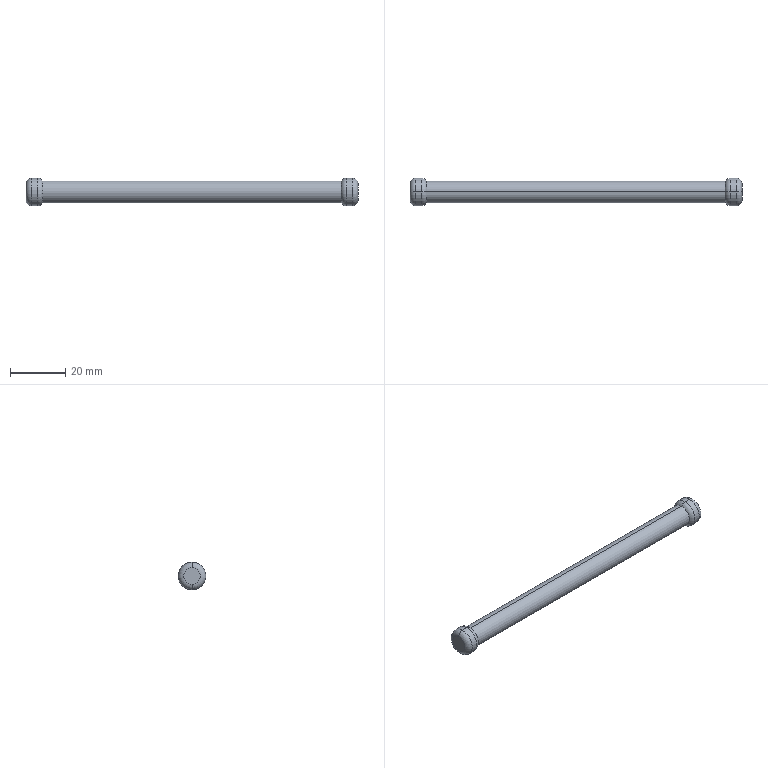Part | SolidWorks | features Fillet 1, ICE 1, MirrorPattern 1, Revolution 1 | 1 solid | 16 faces | box 120 x 10 x 10 mm | volume 6156 mm3 | torus 8 | cylinder 6 | plane 2 | commonest cylinder face diameters 10 x4 7.9 x2
STEP:
#1=CARTESIAN_POINT('',(84.907,0.,-5.));
#2=VERTEX_POINT('',#1);
#3=CARTESIAN_POINT('',(84.907,0.,5.));
#4=VERTEX_POINT('',#3);
#5=CARTESIAN_POINT('',(84.907,0.,0.));
#6=DIRECTION('',(1.,0.,0.));
#7=DIRECTION('',(0.,0.,1.));
#8=AXIS2_PLACEMENT_3D('',#5,#6,#7);
#9=CIRCLE('',#8,5.);
#10=EDGE_CURVE('',#2,#4,#9,.T.);
#11=ORIENTED_EDGE('',*,*,#10,.F.);
#12=CARTESIAN_POINT('',(83.147,0.,-3.95));
#13=VERTEX_POINT('',#12);
#14=CARTESIAN_POINT('',(84.907,0.,-3.));
#15=DIRECTION('',(0.,1.,0.));
#16=DIRECTION('',(0.,0.,1.));
#17=AXIS2_PLACEMENT_3D('',#14,#15,#16);
#18=CIRCLE('',#17,2.);
#19=EDGE_CURVE('',#2,#13,#18,.T.);
#20=ORIENTED_EDGE('',*,*,#19,.T.);
#21=CARTESIAN_POINT('',(83.147,0.,3.95));
#22=VERTEX_POINT('',#21);
#23=CARTESIAN_POINT('',(83.147,0.,0.));
#24=DIRECTION('',(1.,0.,0.));
#25=DIRECTION('',(0.,0.,-1.));
#26=AXIS2_PLACEMENT_3D('',#23,#24,#25);
#27=CIRCLE('',#26,3.95);
#28=EDGE_CURVE('',#13,#22,#27,.T.);
#29=ORIENTED_EDGE('',*,*,#28,.T.);
#30=CARTESIAN_POINT('',(84.907,0.,3.));
#31=DIRECTION('',(0.,-1.,0.));
#32=DIRECTION('',(0.,0.,-1.));
#33=AXIS2_PLACEMENT_3D('',#30,#31,#32);
#34=CIRCLE('',#33,2.);
#35=EDGE_CURVE('',#4,#22,#34,.T.);
#36=ORIENTED_EDGE('',*,*,#35,.F.);
#37=EDGE_LOOP('',(#11,#20,#29,#36));
#38=FACE_OUTER_BOUND('',#37,.T.);
#39=CARTESIAN_POINT('',(84.907,0.,0.));
#40=DIRECTION('',(-1.,0.,0.));
#41=DIRECTION('',(0.,0.,1.));
#42=AXIS2_PLACEMENT_3D('',#39,#40,#41);
#43=TOROIDAL_SURFACE('',#42,3.,2.);
#44=ADVANCED_FACE('',(#38),#43,.T.);
#45=CARTESIAN_POINT('',(89.147,0.,-3.));
#46=VERTEX_POINT('',#45);
#47=CARTESIAN_POINT('',(89.147,0.,3.));
#48=VERTEX_POINT('',#47);
#49=CARTESIAN_POINT('',(89.147,0.,0.));
#50=DIRECTION('',(1.,0.,0.));
#51=DIRECTION('',(0.,0.,1.));
#52=AXIS2_PLACEMENT_3D('',#49,#50,#51);
#53=CIRCLE('',#52,3.);
#54=EDGE_CURVE('',#46,#48,#53,.T.);
#55=ORIENTED_EDGE('',*,*,#54,.F.);
#56=CARTESIAN_POINT('',(87.147,0.,-5.));
#57=VERTEX_POINT('',#56);
#58=CARTESIAN_POINT('',(87.147,0.,-3.));
#59=DIRECTION('',(0.,1.,0.));
#60=DIRECTION('',(0.,0.,1.));
#61=AXIS2_PLACEMENT_3D('',#58,#59,#60);
#62=CIRCLE('',#61,2.);
#63=EDGE_CURVE('',#46,#57,#62,.T.);
#64=ORIENTED_EDGE('',*,*,#63,.T.);
#65=CARTESIAN_POINT('',(87.147,0.,5.));
#66=VERTEX_POINT('',#65);
#67=CARTESIAN_POINT('',(87.147,0.,0.));
#68=DIRECTION('',(-1.,0.,0.));
#69=DIRECTION('',(0.,0.,1.));
#70=AXIS2_PLACEMENT_3D('',#67,#68,#69);
#71=CIRCLE('',#70,5.);
#72=EDGE_CURVE('',#66,#57,#71,.T.);
#73=ORIENTED_EDGE('',*,*,#72,.F.);
#74=CARTESIAN_POINT('',(87.147,0.,3.));
#75=DIRECTION('',(0.,-1.,0.));
#76=DIRECTION('',(0.,0.,-1.));
#77=AXIS2_PLACEMENT_3D('',#74,#75,#76);
#78=CIRCLE('',#77,2.);
#79=EDGE_CURVE('',#48,#66,#78,.T.);
#80=ORIENTED_EDGE('',*,*,#79,.F.);
#81=EDGE_LOOP('',(#55,#64,#73,#80));
#82=FACE_OUTER_BOUND('',#81,.T.);
#83=CARTESIAN_POINT('',(87.147,0.,0.));
#84=DIRECTION('',(-1.,0.,0.));
#85=DIRECTION('',(0.,0.,1.));
#86=AXIS2_PLACEMENT_3D('',#83,#84,#85);
#87=TOROIDAL_SURFACE('',#86,3.,2.);
#88=ADVANCED_FACE('',(#82),#87,.T.);
#89=ORIENTED_EDGE('',*,*,#10,.T.);
#90=CARTESIAN_POINT('',(83.147,0.,5.));
#91=DIRECTION('',(1.,0.,0.));
#92=VECTOR('',#91,1000.);
#93=LINE('',#90,#92);
#94=EDGE_CURVE('',#4,#66,#93,.T.);
#95=ORIENTED_EDGE('',*,*,#94,.T.);
#96=ORIENTED_EDGE('',*,*,#72,.T.);
#97=CARTESIAN_POINT('',(83.147,0.,-5.));
#98=DIRECTION('',(1.,0.,0.));
#99=VECTOR('',#98,1000.);
#100=LINE('',#97,#99);
#101=EDGE_CURVE('',#2,#57,#100,.T.);
#102=ORIENTED_EDGE('',*,*,#101,.F.);
#103=EDGE_LOOP('',(#89,#95,#96,#102));
#104=FACE_OUTER_BOUND('',#103,.T.);
#105=CARTESIAN_POINT('',(83.147,0.,0.));
#106=DIRECTION('',(1.,0.,0.));
#107=DIRECTION('',(0.,0.,-1.));
#108=AXIS2_PLACEMENT_3D('',#105,#106,#107);
#109=CYLINDRICAL_SURFACE('',#108,5.);
#110=ADVANCED_FACE('',(#104),#109,.T.);
#111=CARTESIAN_POINT('',(-26.613,0.,5.));
#112=VERTEX_POINT('',#111);
#113=CARTESIAN_POINT('',(-26.613,0.,-5.));
#114=VERTEX_POINT('',#113);
#115=CARTESIAN_POINT('',(-26.613,0.,0.));
#116=DIRECTION('',(-1.,0.,0.));
#117=DIRECTION('',(0.,0.,-1.));
#118=AXIS2_PLACEMENT_3D('',#115,#116,#117);
#119=CIRCLE('',#118,5.);
#120=EDGE_CURVE('',#112,#114,#119,.T.);
#121=ORIENTED_EDGE('',*,*,#120,.F.);
#122=CARTESIAN_POINT('',(-24.853,0.,3.95));
#123=VERTEX_POINT('',#122);
#124=CARTESIAN_POINT('',(-26.613,0.,3.));
#125=DIRECTION('',(0.,1.,0.));
#126=DIRECTION('',(0.,0.,1.));
#127=AXIS2_PLACEMENT_3D('',#124,#125,#126);
#128=CIRCLE('',#127,2.);
#129=EDGE_CURVE('',#112,#123,#128,.T.);
#130=ORIENTED_EDGE('',*,*,#129,.T.);
#131=CARTESIAN_POINT('',(-24.853,0.,-3.95));
#132=VERTEX_POINT('',#131);
#133=CARTESIAN_POINT('',(-24.853,0.,0.));
#134=DIRECTION('',(-1.,0.,0.));
#135=DIRECTION('',(0.,0.,1.));
#136=AXIS2_PLACEMENT_3D('',#133,#134,#135);
#137=CIRCLE('',#136,3.95);
#138=EDGE_CURVE('',#123,#132,#137,.T.);
#139=ORIENTED_EDGE('',*,*,#138,.T.);
#140=CARTESIAN_POINT('',(-26.613,0.,-3.));
#141=DIRECTION('',(0.,-1.,0.));
#142=DIRECTION('',(0.,0.,-1.));
#143=AXIS2_PLACEMENT_3D('',#140,#141,#142);
#144=CIRCLE('',#143,2.);
#145=EDGE_CURVE('',#114,#132,#144,.T.);
#146=ORIENTED_EDGE('',*,*,#145,.F.);
#147=EDGE_LOOP('',(#121,#130,#139,#146));
#148=FACE_OUTER_BOUND('',#147,.T.);
#149=CARTESIAN_POINT('',(-26.613,0.,0.));
#150=DIRECTION('',(1.,0.,0.));
#151=DIRECTION('',(0.,0.,-1.));
#152=AXIS2_PLACEMENT_3D('',#149,#150,#151);
#153=TOROIDAL_SURFACE('',#152,3.,2.);
#154=ADVANCED_FACE('',(#148),#153,.T.);
#155=CARTESIAN_POINT('',(-30.853,0.,3.));
#156=VERTEX_POINT('',#155);
#157=CARTESIAN_POINT('',(-30.853,0.,-3.));
#158=VERTEX_POINT('',#157);
#159=CARTESIAN_POINT('',(-30.853,0.,0.));
#160=DIRECTION('',(-1.,0.,0.));
#161=DIRECTION('',(0.,0.,-1.));
#162=AXIS2_PLACEMENT_3D('',#159,#160,#161);
#163=CIRCLE('',#162,3.);
#164=EDGE_CURVE('',#156,#158,#163,.T.);
#165=ORIENTED_EDGE('',*,*,#164,.F.);
#166=CARTESIAN_POINT('',(-28.853,0.,5.));
#167=VERTEX_POINT('',#166);
#168=CARTESIAN_POINT('',(-28.853,0.,3.));
#169=DIRECTION('',(0.,1.,0.));
#170=DIRECTION('',(0.,0.,1.));
#171=AXIS2_PLACEMENT_3D('',#168,#169,#170);
#172=CIRCLE('',#171,2.);
#173=EDGE_CURVE('',#156,#167,#172,.T.);
#174=ORIENTED_EDGE('',*,*,#173,.T.);
#175=CARTESIAN_POINT('',(-28.853,0.,-5.));
#176=VERTEX_POINT('',#175);
#177=CARTESIAN_POINT('',(-28.853,0.,0.));
#178=DIRECTION('',(1.,0.,0.));
#179=DIRECTION('',(0.,0.,-1.));
#180=AXIS2_PLACEMENT_3D('',#177,#178,#179);
#181=CIRCLE('',#180,5.);
#182=EDGE_CURVE('',#176,#167,#181,.T.);
#183=ORIENTED_EDGE('',*,*,#182,.F.);
#184=CARTESIAN_POINT('',(-28.853,0.,-3.));
#185=DIRECTION('',(0.,-1.,0.));
#186=DIRECTION('',(0.,0.,-1.));
#187=AXIS2_PLACEMENT_3D('',#184,#185,#186);
#188=CIRCLE('',#187,2.);
#189=EDGE_CURVE('',#158,#176,#188,.T.);
#190=ORIENTED_EDGE('',*,*,#189,.F.);
#191=EDGE_LOOP('',(#165,#174,#183,#190));
#192=FACE_OUTER_BOUND('',#191,.T.);
#193=CARTESIAN_POINT('',(-28.853,0.,0.));
#194=DIRECTION('',(1.,0.,0.));
#195=DIRECTION('',(0.,0.,-1.));
#196=AXIS2_PLACEMENT_3D('',#193,#194,#195);
#197=TOROIDAL_SURFACE('',#196,3.,2.);
#198=ADVANCED_FACE('',(#192),#197,.T.);
#199=ORIENTED_EDGE('',*,*,#120,.T.);
#200=CARTESIAN_POINT('',(-24.853,0.,-5.));
#201=DIRECTION('',(-1.,0.,0.));
#202=VECTOR('',#201,1000.);
#203=LINE('',#200,#202);
#204=EDGE_CURVE('',#114,#176,#203,.T.);
#205=ORIENTED_EDGE('',*,*,#204,.T.);
#206=ORIENTED_EDGE('',*,*,#182,.T.);
#207=CARTESIAN_POINT('',(-24.853,0.,5.));
#208=DIRECTION('',(-1.,0.,0.));
#209=VECTOR('',#208,1000.);
#210=LINE('',#207,#209);
#211=EDGE_CURVE('',#112,#167,#210,.T.);
#212=ORIENTED_EDGE('',*,*,#211,.F.);
#213=EDGE_LOOP('',(#199,#205,#206,#212));
#214=FACE_OUTER_BOUND('',#213,.T.);
#215=CARTESIAN_POINT('',(-24.853,0.,0.));
#216=DIRECTION('',(-1.,0.,0.));
#217=DIRECTION('',(0.,0.,1.));
#218=AXIS2_PLACEMENT_3D('',#215,#216,#217);
#219=CYLINDRICAL_SURFACE('',#218,5.);
#220=ADVANCED_FACE('',(#214),#219,.T.);
#221=ORIENTED_EDGE('',*,*,#28,.F.);
#222=CARTESIAN_POINT('',(-30.853,0.,-3.95));
#223=DIRECTION('',(-1.,0.,0.));
#224=VECTOR('',#223,1000.);
#225=LINE('',#222,#224);
#226=EDGE_CURVE('',#13,#132,#225,.T.);
#227=ORIENTED_EDGE('',*,*,#226,.T.);
#228=ORIENTED_EDGE('',*,*,#138,.F.);
#229=CARTESIAN_POINT('',(-30.853,0.,3.95));
#230=DIRECTION('',(-1.,0.,0.));
#231=VECTOR('',#230,1000.);
#232=LINE('',#229,#231);
#233=EDGE_CURVE('',#22,#123,#232,.T.);
#234=ORIENTED_EDGE('',*,*,#233,.F.);
#235=EDGE_LOOP('',(#221,#227,#228,#234));
#236=FACE_OUTER_BOUND('',#235,.T.);
#237=CARTESIAN_POINT('',(-30.853,0.,0.));
#238=DIRECTION('',(-1.,0.,0.));
#239=DIRECTION('',(0.,0.,1.));
#240=AXIS2_PLACEMENT_3D('',#237,#238,#239);
#241=CYLINDRICAL_SURFACE('',#240,3.95);
#242=ADVANCED_FACE('',(#236),#241,.T.);
#243=ORIENTED_EDGE('',*,*,#226,.F.);
#244=CARTESIAN_POINT('',(83.147,0.,0.));
#245=DIRECTION('',(1.,0.,0.));
#246=DIRECTION('',(0.,0.,-1.));
#247=AXIS2_PLACEMENT_3D('',#244,#245,#246);
#248=CIRCLE('',#247,3.95);
#249=EDGE_CURVE('',#22,#13,#248,.T.);
#250=ORIENTED_EDGE('',*,*,#249,.F.);
#251=ORIENTED_EDGE('',*,*,#233,.T.);
#252=CARTESIAN_POINT('',(-24.853,0.,0.));
#253=DIRECTION('',(-1.,0.,0.));
#254=DIRECTION('',(0.,0.,1.));
#255=AXIS2_PLACEMENT_3D('',#252,#253,#254);
#256=CIRCLE('',#255,3.95);
#257=EDGE_CURVE('',#132,#123,#256,.T.);
#258=ORIENTED_EDGE('',*,*,#257,.F.);
#259=EDGE_LOOP('',(#243,#250,#251,#258));
#260=FACE_OUTER_BOUND('',#259,.T.);
#261=CARTESIAN_POINT('',(-30.853,0.,0.));
#262=DIRECTION('',(-1.,0.,0.));
#263=DIRECTION('',(0.,0.,1.));
#264=AXIS2_PLACEMENT_3D('',#261,#262,#263);
#265=CYLINDRICAL_SURFACE('',#264,3.95);
#266=ADVANCED_FACE('',(#260),#265,.T.);
#267=ORIENTED_EDGE('',*,*,#204,.F.);
#268=CARTESIAN_POINT('',(-26.613,0.,0.));
#269=DIRECTION('',(-1.,0.,0.));
#270=DIRECTION('',(0.,0.,-1.));
#271=AXIS2_PLACEMENT_3D('',#268,#269,#270);
#272=CIRCLE('',#271,5.);
#273=EDGE_CURVE('',#114,#112,#272,.T.);
#274=ORIENTED_EDGE('',*,*,#273,.T.);
#275=ORIENTED_EDGE('',*,*,#211,.T.);
#276=CARTESIAN_POINT('',(-28.853,0.,0.));
#277=DIRECTION('',(1.,0.,0.));
#278=DIRECTION('',(0.,0.,-1.));
#279=AXIS2_PLACEMENT_3D('',#276,#277,#278);
#280=CIRCLE('',#279,5.);
#281=EDGE_CURVE('',#167,#176,#280,.T.);
#282=ORIENTED_EDGE('',*,*,#281,.T.);
#283=EDGE_LOOP('',(#267,#274,#275,#282));
#284=FACE_OUTER_BOUND('',#283,.T.);
#285=CARTESIAN_POINT('',(-24.853,0.,0.));
#286=DIRECTION('',(-1.,0.,0.));
#287=DIRECTION('',(0.,0.,1.));
#288=AXIS2_PLACEMENT_3D('',#285,#286,#287);
#289=CYLINDRICAL_SURFACE('',#288,5.);
#290=ADVANCED_FACE('',(#284),#289,.T.);
#291=CARTESIAN_POINT('',(-30.853,0.,0.));
#292=DIRECTION('',(-1.,0.,0.));
#293=DIRECTION('',(0.,0.,-1.));
#294=AXIS2_PLACEMENT_3D('',#291,#292,#293);
#295=CIRCLE('',#294,3.);
#296=EDGE_CURVE('',#158,#156,#295,.T.);
#297=ORIENTED_EDGE('',*,*,#296,.T.);
#298=ORIENTED_EDGE('',*,*,#164,.T.);
#299=EDGE_LOOP('',(#297,#298));
#300=FACE_OUTER_BOUND('',#299,.T.);
#301=CARTESIAN_POINT('',(-30.853,0.,0.));
#302=DIRECTION('',(1.,0.,0.));
#303=DIRECTION('',(0.,0.,-1.));
#304=AXIS2_PLACEMENT_3D('',#301,#302,#303);
#305=PLANE('',#304);
#306=ADVANCED_FACE('',(#300),#305,.F.);
#307=ORIENTED_EDGE('',*,*,#173,.F.);
#308=ORIENTED_EDGE('',*,*,#296,.F.);
#309=ORIENTED_EDGE('',*,*,#189,.T.);
#310=ORIENTED_EDGE('',*,*,#281,.F.);
#311=EDGE_LOOP('',(#307,#308,#309,#310));
#312=FACE_OUTER_BOUND('',#311,.T.);
#313=CARTESIAN_POINT('',(-28.853,0.,0.));
#314=DIRECTION('',(1.,0.,0.));
#315=DIRECTION('',(0.,0.,-1.));
#316=AXIS2_PLACEMENT_3D('',#313,#314,#315);
#317=TOROIDAL_SURFACE('',#316,3.,2.);
#318=ADVANCED_FACE('',(#312),#317,.T.);
#319=ORIENTED_EDGE('',*,*,#129,.F.);
#320=ORIENTED_EDGE('',*,*,#273,.F.);
#321=ORIENTED_EDGE('',*,*,#145,.T.);
#322=ORIENTED_EDGE('',*,*,#257,.T.);
#323=EDGE_LOOP('',(#319,#320,#321,#322));
#324=FACE_OUTER_BOUND('',#323,.T.);
#325=CARTESIAN_POINT('',(-26.613,0.,0.));
#326=DIRECTION('',(1.,0.,0.));
#327=DIRECTION('',(0.,0.,-1.));
#328=AXIS2_PLACEMENT_3D('',#325,#326,#327);
#329=TOROIDAL_SURFACE('',#328,3.,2.);
#330=ADVANCED_FACE('',(#324),#329,.T.);
#331=ORIENTED_EDGE('',*,*,#94,.F.);
#332=CARTESIAN_POINT('',(84.907,0.,0.));
#333=DIRECTION('',(1.,0.,0.));
#334=DIRECTION('',(0.,0.,1.));
#335=AXIS2_PLACEMENT_3D('',#332,#333,#334);
#336=CIRCLE('',#335,5.);
#337=EDGE_CURVE('',#4,#2,#336,.T.);
#338=ORIENTED_EDGE('',*,*,#337,.T.);
#339=ORIENTED_EDGE('',*,*,#101,.T.);
#340=CARTESIAN_POINT('',(87.147,0.,0.));
#341=DIRECTION('',(-1.,0.,0.));
#342=DIRECTION('',(0.,0.,1.));
#343=AXIS2_PLACEMENT_3D('',#340,#341,#342);
#344=CIRCLE('',#343,5.);
#345=EDGE_CURVE('',#57,#66,#344,.T.);
#346=ORIENTED_EDGE('',*,*,#345,.T.);
#347=EDGE_LOOP('',(#331,#338,#339,#346));
#348=FACE_OUTER_BOUND('',#347,.T.);
#349=CARTESIAN_POINT('',(83.147,0.,0.));
#350=DIRECTION('',(1.,0.,0.));
#351=DIRECTION('',(0.,0.,-1.));
#352=AXIS2_PLACEMENT_3D('',#349,#350,#351);
#353=CYLINDRICAL_SURFACE('',#352,5.);
#354=ADVANCED_FACE('',(#348),#353,.T.);
#355=CARTESIAN_POINT('',(89.147,0.,0.));
#356=DIRECTION('',(1.,0.,0.));
#357=DIRECTION('',(0.,0.,1.));
#358=AXIS2_PLACEMENT_3D('',#355,#356,#357);
#359=CIRCLE('',#358,3.);
#360=EDGE_CURVE('',#48,#46,#359,.T.);
#361=ORIENTED_EDGE('',*,*,#360,.T.);
#362=ORIENTED_EDGE('',*,*,#54,.T.);
#363=EDGE_LOOP('',(#361,#362));
#364=FACE_OUTER_BOUND('',#363,.T.);
#365=CARTESIAN_POINT('',(89.147,3.95,0.));
#366=DIRECTION('',(-1.,0.,0.));
#367=DIRECTION('',(0.,0.,1.));
#368=AXIS2_PLACEMENT_3D('',#365,#366,#367);
#369=PLANE('',#368);
#370=ADVANCED_FACE('',(#364),#369,.F.);
#371=ORIENTED_EDGE('',*,*,#63,.F.);
#372=ORIENTED_EDGE('',*,*,#360,.F.);
#373=ORIENTED_EDGE('',*,*,#79,.T.);
#374=ORIENTED_EDGE('',*,*,#345,.F.);
#375=EDGE_LOOP('',(#371,#372,#373,#374));
#376=FACE_OUTER_BOUND('',#375,.T.);
#377=CARTESIAN_POINT('',(87.147,0.,0.));
#378=DIRECTION('',(-1.,0.,0.));
#379=DIRECTION('',(0.,0.,1.));
#380=AXIS2_PLACEMENT_3D('',#377,#378,#379);
#381=TOROIDAL_SURFACE('',#380,3.,2.);
#382=ADVANCED_FACE('',(#376),#381,.T.);
#383=ORIENTED_EDGE('',*,*,#19,.F.);
#384=ORIENTED_EDGE('',*,*,#337,.F.);
#385=ORIENTED_EDGE('',*,*,#35,.T.);
#386=ORIENTED_EDGE('',*,*,#249,.T.);
#387=EDGE_LOOP('',(#383,#384,#385,#386));
#388=FACE_OUTER_BOUND('',#387,.T.);
#389=CARTESIAN_POINT('',(84.907,0.,0.));
#390=DIRECTION('',(-1.,0.,0.));
#391=DIRECTION('',(0.,0.,1.));
#392=AXIS2_PLACEMENT_3D('',#389,#390,#391);
#393=TOROIDAL_SURFACE('',#392,3.,2.);
#394=ADVANCED_FACE('',(#388),#393,.T.);
#395=CLOSED_SHELL('',(#44,#88,#110,#154,#198,#220,#242,#266,#290,#306,#318,#330,#354,#370,#382,#394));
#396=MANIFOLD_SOLID_BREP('',#395);
#397=CARTESIAN_POINT('',(0.,0.,0.));
#398=DIRECTION('',(0.,0.,1.));
#399=DIRECTION('',(1.,0.,0.));
#400=AXIS2_PLACEMENT_3D('',#397,#398,#399);
#401=(LENGTH_UNIT()NAMED_UNIT(*)SI_UNIT(.MILLI.,.METRE.));
#402=UNCERTAINTY_MEASURE_WITH_UNIT(LENGTH_MEASURE(0.00001),#401,'','');
#403=(NAMED_UNIT(*)PLANE_ANGLE_UNIT()SI_UNIT($,.RADIAN.));
#404=(NAMED_UNIT(*)SI_UNIT($,.STERADIAN.)SOLID_ANGLE_UNIT());
#405=(GEOMETRIC_REPRESENTATION_CONTEXT(3)GLOBAL_UNCERTAINTY_ASSIGNED_CONTEXT((#402))GLOBAL_UNIT_ASSIGNED_CONTEXT((#401,#403,#404))REPRESENTATION_CONTEXT('',''));
#406=ADVANCED_BREP_SHAPE_REPRESENTATION('',(#396,#400),#405);